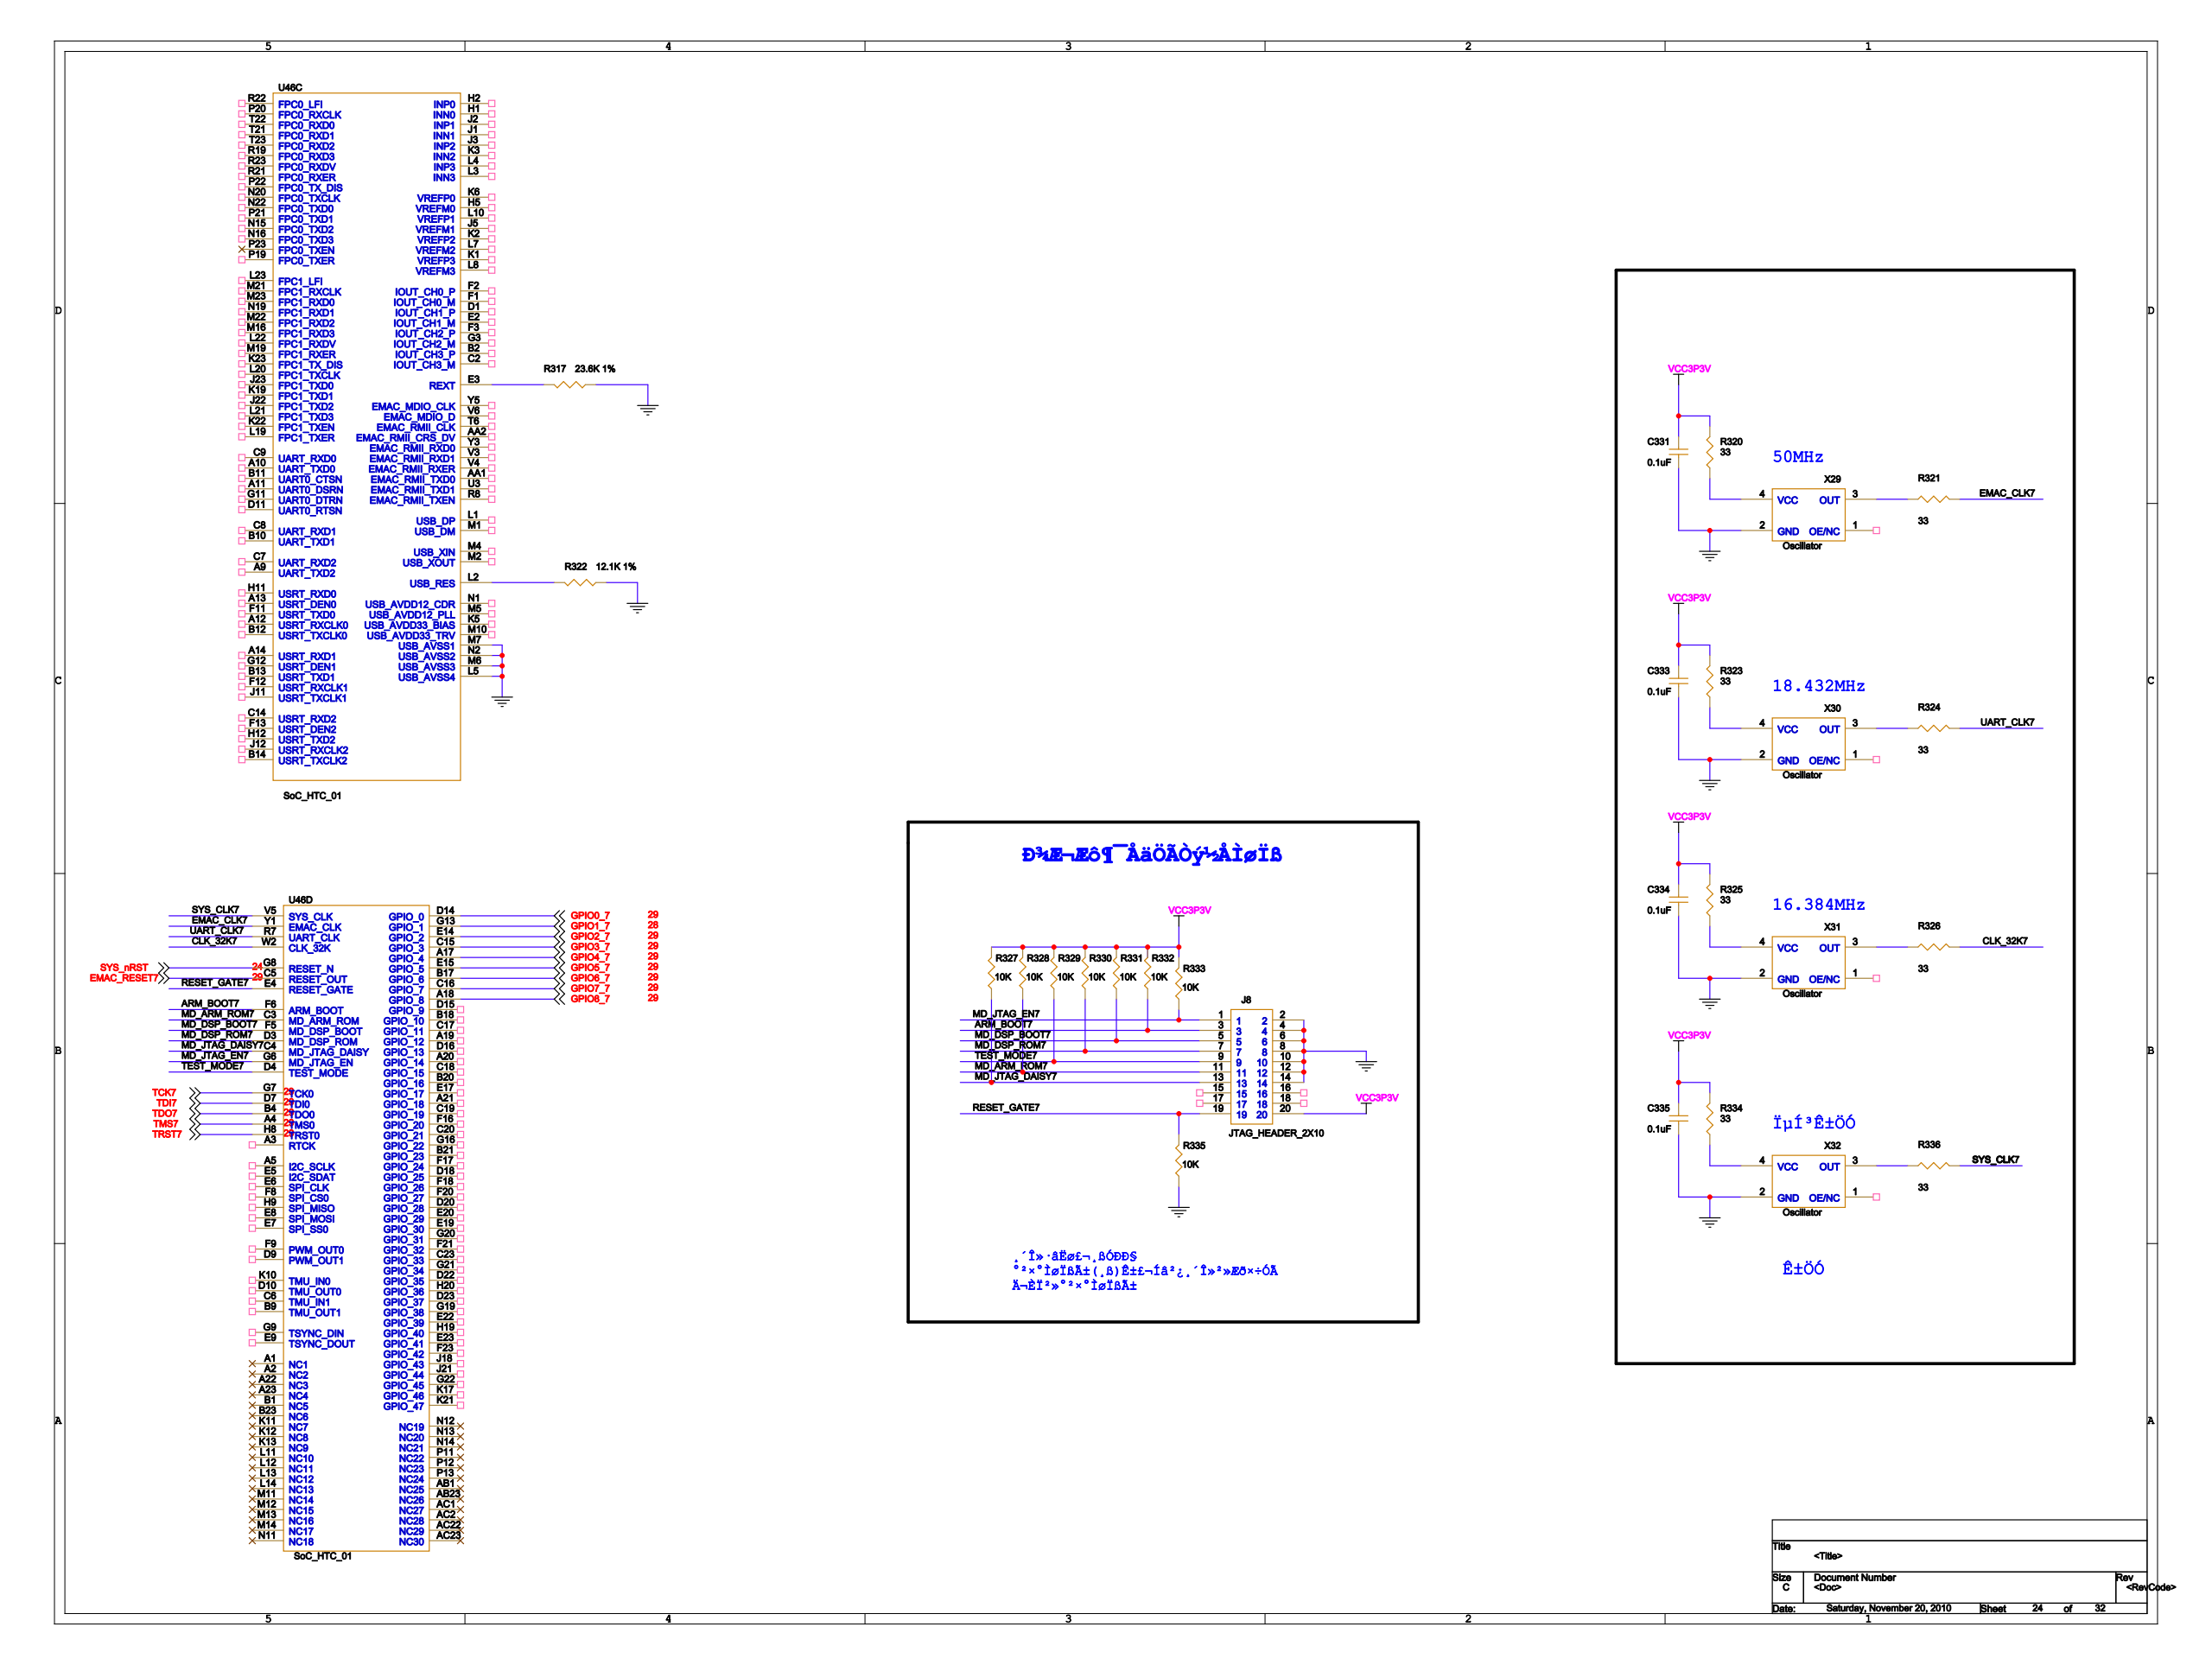Circuit board | Cadence Allegro | 1001 parts | 1318 nets | one sheet of the schematic
Parts on this sheet (reference | value | footprint):
C331 | 0.1uF | 0603
C333 | 0.1uF | 0603
C334 | 0.1uF | 0603
C335 | 0.1uF | 0603
J8 | JTAG_HEADER_2X10 | JTAG_HEADER_2X10
R317 | 23.6K 1% | 0603
R320 | 33 | 0603
R321 | 33 | 0603
R322 | 12.1K 1% | 0603
R323 | 33 | 0603
R324 | 33 | 0603
R325 | 33 | 0603
R326 | 33 | 0603
R327 | 10K | 0603
R328 | 10K | 0603
R329 | 10K | 0603
R330 | 10K | 0603
R331 | 10K | 0603
R332 | 10K | 0603
R333 | 10K | 0603
R334 | 33 | 0603
R335 | 10K | 0603
R336 | 33 | 0603
U46 | SoC_HTC_01 | L529_XIN
X29 | Oscillator | OSC_5_7
X30 | Oscillator | OSC_5_7
X31 | Oscillator | OSC_5_7
X32 | Oscillator | OSC_5_7
Nets of these parts (net: part-pin ...):
GPIO6_7: U46-B17
GPIO8_7: U46-A18
GPIO7_7: U46-C16
GPIO4_7: U46-A17
EMAC_RESET7: U46-C5
TCK7: U46-G7
GPIO1_7: U46-G13
TDO7: U46-B4
GPIO2_7: U46-E14
GPIO0_7: U46-D14
GPIO3_7: U46-C15
GPIO5_7: U46-E15
GND: C331-2 C333-2 C334-2 C335-2 J8-2 J8-4 J8-6 J8-8 J8-10 J8-12 J8-14 R317-1 R322-1 R335-1 X29-2 X30-2 X31-2 X32-2 U46-J8 U46-L5 U46-M6 U46-M7 U46-N2
TMS7: U46-A4
TDI7: U46-D7
TRST7: U46-H8
VCC3P3V: C331-1 C333-1 C334-1 C335-1 J8-20 R320-2 R323-2 R325-2 R327-2 R328-2 R329-2 R330-2 R331-2 R332-2 R333-2 R334-2
N16950065: R317-2 U46-E3
N16950277: R322-2 U46-L2
ARM_BOOT7: J8-3 R332-1 U46-F6
CLK_32K7: R326-2 U46-W2
EMAC_CLK7: R321-2 U46-Y1
MD_ARM_ROM7: J8-11 R328-1 U46-C3
MD_DSP_BOOT7: J8-5 R331-1 U46-F5
MD_DSP_ROM7: J8-7 R330-1 U46-D3
MD_JTAG_DAISY7: J8-13 R327-1 U46-C4
MD_JTAG_EN7: J8-1 R333-1 U46-G6
RESET_GATE7: J8-19 R335-2 U46-E4
SYS_CLK: R336-2 U46-V5
TEST_MODE7: J8-9 R329-1 U46-D4
UART_CLK7: R324-2 U46-R7
N16949632: R320-1 X29-4
N16949608: R321-1 X29-3
N16949622: R323-1 X30-4
N16949640: R324-1 X30-3
N16949818: R325-1 X31-4
N16949848: R326-1 X31-3
N16949829: R334-1 X32-4
N16949876: R336-1 X32-3